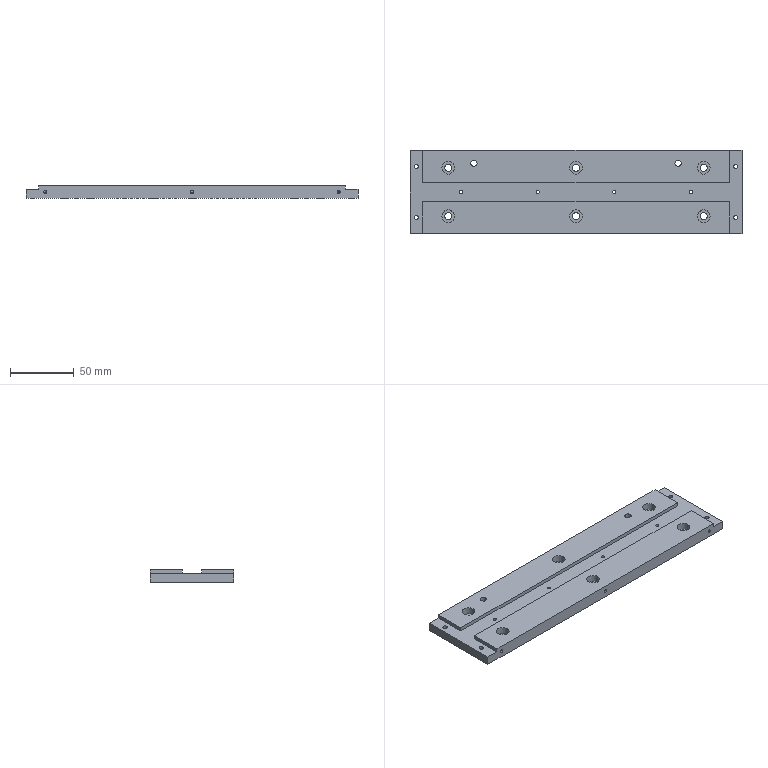Part | STEP file | PN_0061 Mount electronic clip s horizontal manipulator base plate | 1 solid | 76 faces | box 260 x 65 x 10 mm | volume 150103 mm3 | cylinder 50 | plane 20 | cone 6 | commonest cylinder face diameters 2.5 x14 5.5 x12 10 x12 3.3 x8 5 x4